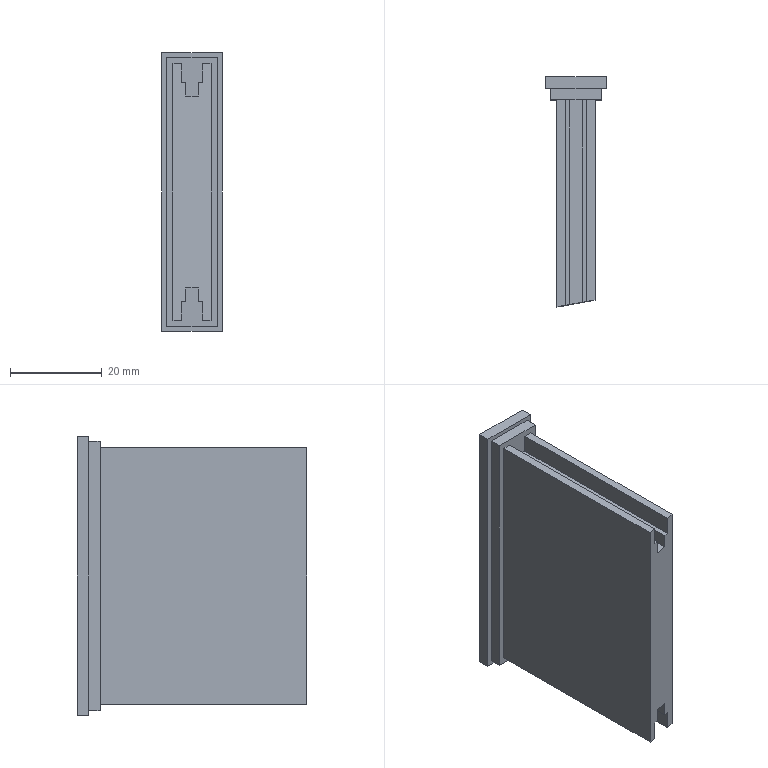Part | SolidWorks | features ICE 3, Extrusion 1 | 1 solid | 32 faces | box 13.06 x 50 x 60.56 mm | volume 21649 mm3 | plane 32
STEP:
#1=CARTESIAN_POINT('',(-2.36,45.,-27.89));
#2=VERTEX_POINT('',#1);
#3=CARTESIAN_POINT('',(-2.36,0.3139,-27.89));
#4=VERTEX_POINT('',#3);
#5=CARTESIAN_POINT('',(-2.36,45.,-27.89));
#6=DIRECTION('',(0.,-1.,0.));
#7=VECTOR('',#6,1000.);
#8=LINE('',#5,#7);
#9=EDGE_CURVE('',#2,#4,#8,.T.);
#10=ORIENTED_EDGE('',*,*,#9,.T.);
#11=CARTESIAN_POINT('',(-4.14,0.,-27.89));
#12=VERTEX_POINT('',#11);
#13=CARTESIAN_POINT('',(4.14,1.46,-27.89));
#14=DIRECTION('',(-0.9848,-0.1736,0.));
#15=VECTOR('',#14,1000.);
#16=LINE('',#13,#15);
#17=EDGE_CURVE('',#4,#12,#16,.T.);
#18=ORIENTED_EDGE('',*,*,#17,.T.);
#19=CARTESIAN_POINT('',(-4.14,45.,-27.89));
#20=VERTEX_POINT('',#19);
#21=CARTESIAN_POINT('',(-4.14,45.,-27.89));
#22=DIRECTION('',(0.,-1.,0.));
#23=VECTOR('',#22,1000.);
#24=LINE('',#21,#23);
#25=EDGE_CURVE('',#20,#12,#24,.T.);
#26=ORIENTED_EDGE('',*,*,#25,.F.);
#27=CARTESIAN_POINT('',(-2.36,45.,-27.89));
#28=DIRECTION('',(-1.,0.,0.));
#29=VECTOR('',#28,1000.);
#30=LINE('',#27,#29);
#31=EDGE_CURVE('',#2,#20,#30,.T.);
#32=ORIENTED_EDGE('',*,*,#31,.F.);
#33=EDGE_LOOP('',(#10,#18,#26,#32));
#34=FACE_OUTER_BOUND('',#33,.T.);
#35=CARTESIAN_POINT('',(-2.36,45.,-27.89));
#36=DIRECTION('',(0.,0.,1.));
#37=DIRECTION('',(1.,0.,0.));
#38=AXIS2_PLACEMENT_3D('',#35,#36,#37);
#39=PLANE('',#38);
#40=ADVANCED_FACE('',(#34),#39,.F.);
#41=CARTESIAN_POINT('',(-4.14,0.,27.89));
#42=VERTEX_POINT('',#41);
#43=CARTESIAN_POINT('',(-4.14,0.,-27.89));
#44=DIRECTION('',(0.,0.,1.));
#45=VECTOR('',#44,1000.);
#46=LINE('',#43,#45);
#47=EDGE_CURVE('',#12,#42,#46,.T.);
#48=ORIENTED_EDGE('',*,*,#47,.T.);
#49=CARTESIAN_POINT('',(-4.14,45.,27.89));
#50=VERTEX_POINT('',#49);
#51=CARTESIAN_POINT('',(-4.14,45.,27.89));
#52=DIRECTION('',(0.,-1.,0.));
#53=VECTOR('',#52,1000.);
#54=LINE('',#51,#53);
#55=EDGE_CURVE('',#50,#42,#54,.T.);
#56=ORIENTED_EDGE('',*,*,#55,.F.);
#57=CARTESIAN_POINT('',(-4.14,45.,-27.89));
#58=DIRECTION('',(0.,0.,1.));
#59=VECTOR('',#58,1000.);
#60=LINE('',#57,#59);
#61=EDGE_CURVE('',#20,#50,#60,.T.);
#62=ORIENTED_EDGE('',*,*,#61,.F.);
#63=ORIENTED_EDGE('',*,*,#25,.T.);
#64=EDGE_LOOP('',(#48,#56,#62,#63));
#65=FACE_OUTER_BOUND('',#64,.T.);
#66=CARTESIAN_POINT('',(-4.14,45.,-27.89));
#67=DIRECTION('',(1.,0.,0.));
#68=DIRECTION('',(0.,0.,-1.));
#69=AXIS2_PLACEMENT_3D('',#66,#67,#68);
#70=PLANE('',#69);
#71=ADVANCED_FACE('',(#65),#70,.F.);
#72=ORIENTED_EDGE('',*,*,#55,.T.);
#73=CARTESIAN_POINT('',(-2.36,0.3139,27.89));
#74=VERTEX_POINT('',#73);
#75=CARTESIAN_POINT('',(4.14,1.46,27.89));
#76=DIRECTION('',(-0.9848,-0.1736,0.));
#77=VECTOR('',#76,1000.);
#78=LINE('',#75,#77);
#79=EDGE_CURVE('',#74,#42,#78,.T.);
#80=ORIENTED_EDGE('',*,*,#79,.F.);
#81=CARTESIAN_POINT('',(-2.36,45.,27.89));
#82=VERTEX_POINT('',#81);
#83=CARTESIAN_POINT('',(-2.36,45.,27.89));
#84=DIRECTION('',(0.,-1.,0.));
#85=VECTOR('',#84,1000.);
#86=LINE('',#83,#85);
#87=EDGE_CURVE('',#82,#74,#86,.T.);
#88=ORIENTED_EDGE('',*,*,#87,.F.);
#89=CARTESIAN_POINT('',(-4.14,45.,27.89));
#90=DIRECTION('',(1.,0.,0.));
#91=VECTOR('',#90,1000.);
#92=LINE('',#89,#91);
#93=EDGE_CURVE('',#50,#82,#92,.T.);
#94=ORIENTED_EDGE('',*,*,#93,.F.);
#95=EDGE_LOOP('',(#72,#80,#88,#94));
#96=FACE_OUTER_BOUND('',#95,.T.);
#97=CARTESIAN_POINT('',(-4.14,45.,27.89));
#98=DIRECTION('',(0.,0.,-1.));
#99=DIRECTION('',(-1.,0.,0.));
#100=AXIS2_PLACEMENT_3D('',#97,#98,#99);
#101=PLANE('',#100);
#102=ADVANCED_FACE('',(#96),#101,.F.);
#103=ORIENTED_EDGE('',*,*,#87,.T.);
#104=CARTESIAN_POINT('',(-2.36,0.3139,23.89));
#105=VERTEX_POINT('',#104);
#106=CARTESIAN_POINT('',(-2.36,0.3139,27.89));
#107=DIRECTION('',(0.,0.,-1.));
#108=VECTOR('',#107,1000.);
#109=LINE('',#106,#108);
#110=EDGE_CURVE('',#74,#105,#109,.T.);
#111=ORIENTED_EDGE('',*,*,#110,.T.);
#112=CARTESIAN_POINT('',(-2.36,45.,23.89));
#113=VERTEX_POINT('',#112);
#114=CARTESIAN_POINT('',(-2.36,45.,23.89));
#115=DIRECTION('',(0.,-1.,0.));
#116=VECTOR('',#115,1000.);
#117=LINE('',#114,#116);
#118=EDGE_CURVE('',#113,#105,#117,.T.);
#119=ORIENTED_EDGE('',*,*,#118,.F.);
#120=CARTESIAN_POINT('',(-2.36,45.,27.89));
#121=DIRECTION('',(0.,0.,-1.));
#122=VECTOR('',#121,1000.);
#123=LINE('',#120,#122);
#124=EDGE_CURVE('',#82,#113,#123,.T.);
#125=ORIENTED_EDGE('',*,*,#124,.F.);
#126=EDGE_LOOP('',(#103,#111,#119,#125));
#127=FACE_OUTER_BOUND('',#126,.T.);
#128=CARTESIAN_POINT('',(-2.36,45.,27.89));
#129=DIRECTION('',(-1.,0.,0.));
#130=DIRECTION('',(0.,0.,1.));
#131=AXIS2_PLACEMENT_3D('',#128,#129,#130);
#132=PLANE('',#131);
#133=ADVANCED_FACE('',(#127),#132,.F.);
#134=ORIENTED_EDGE('',*,*,#118,.T.);
#135=CARTESIAN_POINT('',(-1.36,0.4902,23.89));
#136=VERTEX_POINT('',#135);
#137=CARTESIAN_POINT('',(5.282,1.661,23.89));
#138=DIRECTION('',(0.9848,0.1736,0.));
#139=VECTOR('',#138,1000.);
#140=LINE('',#137,#139);
#141=EDGE_CURVE('',#105,#136,#140,.T.);
#142=ORIENTED_EDGE('',*,*,#141,.T.);
#143=CARTESIAN_POINT('',(-1.36,45.,23.89));
#144=VERTEX_POINT('',#143);
#145=CARTESIAN_POINT('',(-1.36,45.,23.89));
#146=DIRECTION('',(0.,-1.,0.));
#147=VECTOR('',#146,1000.);
#148=LINE('',#145,#147);
#149=EDGE_CURVE('',#144,#136,#148,.T.);
#150=ORIENTED_EDGE('',*,*,#149,.F.);
#151=CARTESIAN_POINT('',(-2.36,45.,23.89));
#152=DIRECTION('',(1.,0.,0.));
#153=VECTOR('',#152,1000.);
#154=LINE('',#151,#153);
#155=EDGE_CURVE('',#113,#144,#154,.T.);
#156=ORIENTED_EDGE('',*,*,#155,.F.);
#157=EDGE_LOOP('',(#134,#142,#150,#156));
#158=FACE_OUTER_BOUND('',#157,.T.);
#159=CARTESIAN_POINT('',(-2.36,45.,23.89));
#160=DIRECTION('',(0.,0.,-1.));
#161=DIRECTION('',(-1.,0.,0.));
#162=AXIS2_PLACEMENT_3D('',#159,#160,#161);
#163=PLANE('',#162);
#164=ADVANCED_FACE('',(#158),#163,.F.);
#165=ORIENTED_EDGE('',*,*,#149,.T.);
#166=CARTESIAN_POINT('',(-1.36,0.4902,20.89));
#167=VERTEX_POINT('',#166);
#168=CARTESIAN_POINT('',(-1.36,0.4902,23.89));
#169=DIRECTION('',(0.,0.,-1.));
#170=VECTOR('',#169,1000.);
#171=LINE('',#168,#170);
#172=EDGE_CURVE('',#136,#167,#171,.T.);
#173=ORIENTED_EDGE('',*,*,#172,.T.);
#174=CARTESIAN_POINT('',(-1.36,45.,20.89));
#175=VERTEX_POINT('',#174);
#176=CARTESIAN_POINT('',(-1.36,45.,20.89));
#177=DIRECTION('',(0.,-1.,0.));
#178=VECTOR('',#177,1000.);
#179=LINE('',#176,#178);
#180=EDGE_CURVE('',#175,#167,#179,.T.);
#181=ORIENTED_EDGE('',*,*,#180,.F.);
#182=CARTESIAN_POINT('',(-1.36,45.,23.89));
#183=DIRECTION('',(0.,0.,-1.));
#184=VECTOR('',#183,1000.);
#185=LINE('',#182,#184);
#186=EDGE_CURVE('',#144,#175,#185,.T.);
#187=ORIENTED_EDGE('',*,*,#186,.F.);
#188=EDGE_LOOP('',(#165,#173,#181,#187));
#189=FACE_OUTER_BOUND('',#188,.T.);
#190=CARTESIAN_POINT('',(-1.36,45.,23.89));
#191=DIRECTION('',(-1.,0.,0.));
#192=DIRECTION('',(0.,0.,1.));
#193=AXIS2_PLACEMENT_3D('',#190,#191,#192);
#194=PLANE('',#193);
#195=ADVANCED_FACE('',(#189),#194,.F.);
#196=ORIENTED_EDGE('',*,*,#180,.T.);
#197=CARTESIAN_POINT('',(1.36,0.9698,20.89));
#198=VERTEX_POINT('',#197);
#199=CARTESIAN_POINT('',(6.252,1.832,20.89));
#200=DIRECTION('',(0.9848,0.1736,0.));
#201=VECTOR('',#200,1000.);
#202=LINE('',#199,#201);
#203=EDGE_CURVE('',#167,#198,#202,.T.);
#204=ORIENTED_EDGE('',*,*,#203,.T.);
#205=CARTESIAN_POINT('',(1.36,45.,20.89));
#206=VERTEX_POINT('',#205);
#207=CARTESIAN_POINT('',(1.36,45.,20.89));
#208=DIRECTION('',(0.,-1.,0.));
#209=VECTOR('',#208,1000.);
#210=LINE('',#207,#209);
#211=EDGE_CURVE('',#206,#198,#210,.T.);
#212=ORIENTED_EDGE('',*,*,#211,.F.);
#213=CARTESIAN_POINT('',(-1.36,45.,20.89));
#214=DIRECTION('',(1.,0.,0.));
#215=VECTOR('',#214,1000.);
#216=LINE('',#213,#215);
#217=EDGE_CURVE('',#175,#206,#216,.T.);
#218=ORIENTED_EDGE('',*,*,#217,.F.);
#219=EDGE_LOOP('',(#196,#204,#212,#218));
#220=FACE_OUTER_BOUND('',#219,.T.);
#221=CARTESIAN_POINT('',(-1.36,45.,20.89));
#222=DIRECTION('',(0.,0.,-1.));
#223=DIRECTION('',(-1.,0.,0.));
#224=AXIS2_PLACEMENT_3D('',#221,#222,#223);
#225=PLANE('',#224);
#226=ADVANCED_FACE('',(#220),#225,.F.);
#227=ORIENTED_EDGE('',*,*,#211,.T.);
#228=CARTESIAN_POINT('',(1.36,0.9698,23.89));
#229=VERTEX_POINT('',#228);
#230=CARTESIAN_POINT('',(1.36,0.9698,20.89));
#231=DIRECTION('',(0.,0.,1.));
#232=VECTOR('',#231,1000.);
#233=LINE('',#230,#232);
#234=EDGE_CURVE('',#198,#229,#233,.T.);
#235=ORIENTED_EDGE('',*,*,#234,.T.);
#236=CARTESIAN_POINT('',(1.36,45.,23.89));
#237=VERTEX_POINT('',#236);
#238=CARTESIAN_POINT('',(1.36,45.,23.89));
#239=DIRECTION('',(0.,-1.,0.));
#240=VECTOR('',#239,1000.);
#241=LINE('',#238,#240);
#242=EDGE_CURVE('',#237,#229,#241,.T.);
#243=ORIENTED_EDGE('',*,*,#242,.F.);
#244=CARTESIAN_POINT('',(1.36,45.,20.89));
#245=DIRECTION('',(0.,0.,1.));
#246=VECTOR('',#245,1000.);
#247=LINE('',#244,#246);
#248=EDGE_CURVE('',#206,#237,#247,.T.);
#249=ORIENTED_EDGE('',*,*,#248,.F.);
#250=EDGE_LOOP('',(#227,#235,#243,#249));
#251=FACE_OUTER_BOUND('',#250,.T.);
#252=CARTESIAN_POINT('',(1.36,45.,20.89));
#253=DIRECTION('',(1.,0.,0.));
#254=DIRECTION('',(0.,0.,-1.));
#255=AXIS2_PLACEMENT_3D('',#252,#253,#254);
#256=PLANE('',#255);
#257=ADVANCED_FACE('',(#251),#256,.F.);
#258=ORIENTED_EDGE('',*,*,#242,.T.);
#259=CARTESIAN_POINT('',(2.36,1.146,23.89));
#260=VERTEX_POINT('',#259);
#261=CARTESIAN_POINT('',(8.89,2.297,23.89));
#262=DIRECTION('',(0.9848,0.1736,0.));
#263=VECTOR('',#262,1000.);
#264=LINE('',#261,#263);
#265=EDGE_CURVE('',#229,#260,#264,.T.);
#266=ORIENTED_EDGE('',*,*,#265,.T.);
#267=CARTESIAN_POINT('',(2.36,45.,23.89));
#268=VERTEX_POINT('',#267);
#269=CARTESIAN_POINT('',(2.36,45.,23.89));
#270=DIRECTION('',(0.,-1.,0.));
#271=VECTOR('',#270,1000.);
#272=LINE('',#269,#271);
#273=EDGE_CURVE('',#268,#260,#272,.T.);
#274=ORIENTED_EDGE('',*,*,#273,.F.);
#275=CARTESIAN_POINT('',(1.36,45.,23.89));
#276=DIRECTION('',(1.,0.,0.));
#277=VECTOR('',#276,1000.);
#278=LINE('',#275,#277);
#279=EDGE_CURVE('',#237,#268,#278,.T.);
#280=ORIENTED_EDGE('',*,*,#279,.F.);
#281=EDGE_LOOP('',(#258,#266,#274,#280));
#282=FACE_OUTER_BOUND('',#281,.T.);
#283=CARTESIAN_POINT('',(1.36,45.,23.89));
#284=DIRECTION('',(0.,0.,-1.));
#285=DIRECTION('',(-1.,0.,0.));
#286=AXIS2_PLACEMENT_3D('',#283,#284,#285);
#287=PLANE('',#286);
#288=ADVANCED_FACE('',(#282),#287,.F.);
#289=ORIENTED_EDGE('',*,*,#273,.T.);
#290=CARTESIAN_POINT('',(2.36,1.146,27.89));
#291=VERTEX_POINT('',#290);
#292=CARTESIAN_POINT('',(2.36,1.146,23.89));
#293=DIRECTION('',(0.,0.,1.));
#294=VECTOR('',#293,1000.);
#295=LINE('',#292,#294);
#296=EDGE_CURVE('',#260,#291,#295,.T.);
#297=ORIENTED_EDGE('',*,*,#296,.T.);
#298=CARTESIAN_POINT('',(2.36,45.,27.89));
#299=VERTEX_POINT('',#298);
#300=CARTESIAN_POINT('',(2.36,45.,27.89));
#301=DIRECTION('',(0.,-1.,0.));
#302=VECTOR('',#301,1000.);
#303=LINE('',#300,#302);
#304=EDGE_CURVE('',#299,#291,#303,.T.);
#305=ORIENTED_EDGE('',*,*,#304,.F.);
#306=CARTESIAN_POINT('',(2.36,45.,23.89));
#307=DIRECTION('',(0.,0.,1.));
#308=VECTOR('',#307,1000.);
#309=LINE('',#306,#308);
#310=EDGE_CURVE('',#268,#299,#309,.T.);
#311=ORIENTED_EDGE('',*,*,#310,.F.);
#312=EDGE_LOOP('',(#289,#297,#305,#311));
#313=FACE_OUTER_BOUND('',#312,.T.);
#314=CARTESIAN_POINT('',(2.36,45.,23.89));
#315=DIRECTION('',(1.,0.,0.));
#316=DIRECTION('',(0.,0.,-1.));
#317=AXIS2_PLACEMENT_3D('',#314,#315,#316);
#318=PLANE('',#317);
#319=ADVANCED_FACE('',(#313),#318,.F.);
#320=ORIENTED_EDGE('',*,*,#304,.T.);
#321=CARTESIAN_POINT('',(4.14,1.46,27.89));
#322=VERTEX_POINT('',#321);
#323=CARTESIAN_POINT('',(4.14,1.46,27.89));
#324=DIRECTION('',(-0.9848,-0.1736,0.));
#325=VECTOR('',#324,1000.);
#326=LINE('',#323,#325);
#327=EDGE_CURVE('',#322,#291,#326,.T.);
#328=ORIENTED_EDGE('',*,*,#327,.F.);
#329=CARTESIAN_POINT('',(4.14,45.,27.89));
#330=VERTEX_POINT('',#329);
#331=CARTESIAN_POINT('',(4.14,45.,27.89));
#332=DIRECTION('',(0.,-1.,0.));
#333=VECTOR('',#332,1000.);
#334=LINE('',#331,#333);
#335=EDGE_CURVE('',#330,#322,#334,.T.);
#336=ORIENTED_EDGE('',*,*,#335,.F.);
#337=CARTESIAN_POINT('',(2.36,45.,27.89));
#338=DIRECTION('',(1.,0.,0.));
#339=VECTOR('',#338,1000.);
#340=LINE('',#337,#339);
#341=EDGE_CURVE('',#299,#330,#340,.T.);
#342=ORIENTED_EDGE('',*,*,#341,.F.);
#343=EDGE_LOOP('',(#320,#328,#336,#342));
#344=FACE_OUTER_BOUND('',#343,.T.);
#345=CARTESIAN_POINT('',(2.36,45.,27.89));
#346=DIRECTION('',(0.,0.,-1.));
#347=DIRECTION('',(-1.,0.,0.));
#348=AXIS2_PLACEMENT_3D('',#345,#346,#347);
#349=PLANE('',#348);
#350=ADVANCED_FACE('',(#344),#349,.F.);
#351=ORIENTED_EDGE('',*,*,#335,.T.);
#352=CARTESIAN_POINT('',(4.14,1.46,-27.89));
#353=VERTEX_POINT('',#352);
#354=CARTESIAN_POINT('',(4.14,1.46,-27.89));
#355=DIRECTION('',(0.,0.,1.));
#356=VECTOR('',#355,1000.);
#357=LINE('',#354,#356);
#358=EDGE_CURVE('',#353,#322,#357,.T.);
#359=ORIENTED_EDGE('',*,*,#358,.F.);
#360=CARTESIAN_POINT('',(4.14,45.,-27.89));
#361=VERTEX_POINT('',#360);
#362=CARTESIAN_POINT('',(4.14,45.,-27.89));
#363=DIRECTION('',(0.,-1.,0.));
#364=VECTOR('',#363,1000.);
#365=LINE('',#362,#364);
#366=EDGE_CURVE('',#361,#353,#365,.T.);
#367=ORIENTED_EDGE('',*,*,#366,.F.);
#368=CARTESIAN_POINT('',(4.14,45.,27.89));
#369=DIRECTION('',(0.,0.,-1.));
#370=VECTOR('',#369,1000.);
#371=LINE('',#368,#370);
#372=EDGE_CURVE('',#330,#361,#371,.T.);
#373=ORIENTED_EDGE('',*,*,#372,.F.);
#374=EDGE_LOOP('',(#351,#359,#367,#373));
#375=FACE_OUTER_BOUND('',#374,.T.);
#376=CARTESIAN_POINT('',(4.14,45.,27.89));
#377=DIRECTION('',(-1.,0.,0.));
#378=DIRECTION('',(0.,0.,1.));
#379=AXIS2_PLACEMENT_3D('',#376,#377,#378);
#380=PLANE('',#379);
#381=ADVANCED_FACE('',(#375),#380,.F.);
#382=ORIENTED_EDGE('',*,*,#366,.T.);
#383=CARTESIAN_POINT('',(2.36,1.146,-27.89));
#384=VERTEX_POINT('',#383);
#385=CARTESIAN_POINT('',(4.14,1.46,-27.89));
#386=DIRECTION('',(-0.9848,-0.1736,0.));
#387=VECTOR('',#386,1000.);
#388=LINE('',#385,#387);
#389=EDGE_CURVE('',#353,#384,#388,.T.);
#390=ORIENTED_EDGE('',*,*,#389,.T.);
#391=CARTESIAN_POINT('',(2.36,45.,-27.89));
#392=VERTEX_POINT('',#391);
#393=CARTESIAN_POINT('',(2.36,45.,-27.89));
#394=DIRECTION('',(0.,-1.,0.));
#395=VECTOR('',#394,1000.);
#396=LINE('',#393,#395);
#397=EDGE_CURVE('',#392,#384,#396,.T.);
#398=ORIENTED_EDGE('',*,*,#397,.F.);
#399=CARTESIAN_POINT('',(4.14,45.,-27.89));
#400=DIRECTION('',(-1.,0.,0.));
#401=VECTOR('',#400,1000.);
#402=LINE('',#399,#401);
#403=EDGE_CURVE('',#361,#392,#402,.T.);
#404=ORIENTED_EDGE('',*,*,#403,.F.);
#405=EDGE_LOOP('',(#382,#390,#398,#404));
#406=FACE_OUTER_BOUND('',#405,.T.);
#407=CARTESIAN_POINT('',(4.14,45.,-27.89));
#408=DIRECTION('',(0.,0.,1.));
#409=DIRECTION('',(1.,0.,0.));
#410=AXIS2_PLACEMENT_3D('',#407,#408,#409);
#411=PLANE('',#410);
#412=ADVANCED_FACE('',(#406),#411,.F.);
#413=ORIENTED_EDGE('',*,*,#397,.T.);
#414=CARTESIAN_POINT('',(2.36,1.146,-23.89));
#415=VERTEX_POINT('',#414);
#416=CARTESIAN_POINT('',(2.36,1.146,-27.89));
#417=DIRECTION('',(0.,0.,1.));
#418=VECTOR('',#417,1000.);
#419=LINE('',#416,#418);
#420=EDGE_CURVE('',#384,#415,#419,.T.);
#421=ORIENTED_EDGE('',*,*,#420,.T.);
#422=CARTESIAN_POINT('',(2.36,45.,-23.89));
#423=VERTEX_POINT('',#422);
#424=CARTESIAN_POINT('',(2.36,45.,-23.89));
#425=DIRECTION('',(0.,-1.,0.));
#426=VECTOR('',#425,1000.);
#427=LINE('',#424,#426);
#428=EDGE_CURVE('',#423,#415,#427,.T.);
#429=ORIENTED_EDGE('',*,*,#428,.F.);
#430=CARTESIAN_POINT('',(2.36,45.,-27.89));
#431=DIRECTION('',(0.,0.,1.));
#432=VECTOR('',#431,1000.);
#433=LINE('',#430,#432);
#434=EDGE_CURVE('',#392,#423,#433,.T.);
#435=ORIENTED_EDGE('',*,*,#434,.F.);
#436=EDGE_LOOP('',(#413,#421,#429,#435));
#437=FACE_OUTER_BOUND('',#436,.T.);
#438=CARTESIAN_POINT('',(2.36,45.,-27.89));
#439=DIRECTION('',(1.,0.,0.));
#440=DIRECTION('',(0.,0.,-1.));
#441=AXIS2_PLACEMENT_3D('',#438,#439,#440);
#442=PLANE('',#441);
#443=ADVANCED_FACE('',(#437),#442,.F.);
#444=ORIENTED_EDGE('',*,*,#428,.T.);
#445=CARTESIAN_POINT('',(1.36,0.9698,-23.89));
#446=VERTEX_POINT('',#445);
#447=CARTESIAN_POINT('',(9.859,2.468,-23.89));
#448=DIRECTION('',(-0.9848,-0.1736,0.));
#449=VECTOR('',#448,1000.);
#450=LINE('',#447,#449);
#451=EDGE_CURVE('',#415,#446,#450,.T.);
#452=ORIENTED_EDGE('',*,*,#451,.T.);
#453=CARTESIAN_POINT('',(1.36,45.,-23.89));
#454=VERTEX_POINT('',#453);
#455=CARTESIAN_POINT('',(1.36,45.,-23.89));
#456=DIRECTION('',(0.,-1.,0.));
#457=VECTOR('',#456,1000.);
#458=LINE('',#455,#457);
#459=EDGE_CURVE('',#454,#446,#458,.T.);
#460=ORIENTED_EDGE('',*,*,#459,.F.);
#461=CARTESIAN_POINT('',(2.36,45.,-23.89));
#462=DIRECTION('',(-1.,0.,0.));
#463=VECTOR('',#462,1000.);
#464=LINE('',#461,#463);
#465=EDGE_CURVE('',#423,#454,#464,.T.);
#466=ORIENTED_EDGE('',*,*,#465,.F.);
#467=EDGE_LOOP('',(#444,#452,#460,#466));
#468=FACE_OUTER_BOUND('',#467,.T.);
#469=CARTESIAN_POINT('',(2.36,45.,-23.89));
#470=DIRECTION('',(0.,0.,1.));
#471=DIRECTION('',(1.,0.,0.));
#472=AXIS2_PLACEMENT_3D('',#469,#470,#471);
#473=PLANE('',#472);
#474=ADVANCED_FACE('',(#468),#473,.F.);
#475=ORIENTED_EDGE('',*,*,#459,.T.);
#476=CARTESIAN_POINT('',(1.36,0.9698,-20.89));
#477=VERTEX_POINT('',#476);
#478=CARTESIAN_POINT('',(1.36,0.9698,-23.89));
#479=DIRECTION('',(0.,0.,1.));
#480=VECTOR('',#479,1000.);
#481=LINE('',#478,#480);
#482=EDGE_CURVE('',#446,#477,#481,.T.);
#483=ORIENTED_EDGE('',*,*,#482,.T.);
#484=CARTESIAN_POINT('',(1.36,45.,-20.89));
#485=VERTEX_POINT('',#484);
#486=CARTESIAN_POINT('',(1.36,45.,-20.89));
#487=DIRECTION('',(0.,-1.,0.));
#488=VECTOR('',#487,1000.);
#489=LINE('',#486,#488);
#490=EDGE_CURVE('',#485,#477,#489,.T.);
#491=ORIENTED_EDGE('',*,*,#490,.F.);
#492=CARTESIAN_POINT('',(1.36,45.,-23.89));
#493=DIRECTION('',(0.,0.,1.));
#494=VECTOR('',#493,1000.);
#495=LINE('',#492,#494);
#496=EDGE_CURVE('',#454,#485,#495,.T.);
#497=ORIENTED_EDGE('',*,*,#496,.F.);
#498=EDGE_LOOP('',(#475,#483,#491,#497));
#499=FACE_OUTER_BOUND('',#498,.T.);
#500=CARTESIAN_POINT('',(1.36,45.,-23.89));
#501=DIRECTION('',(1.,0.,0.));
#502=DIRECTION('',(0.,0.,-1.));
#503=AXIS2_PLACEMENT_3D('',#500,#501,#502);
#504=PLANE('',#503);
#505=ADVANCED_FACE('',(#499),#504,.F.);
#506=ORIENTED_EDGE('',*,*,#490,.T.);
#507=CARTESIAN_POINT('',(-1.36,0.4902,-20.89));
#508=VERTEX_POINT('',#507);
#509=CARTESIAN_POINT('',(8.89,2.297,-20.89));
#510=DIRECTION('',(-0.9848,-0.1736,0.));
#511=VECTOR('',#510,1000.);
#512=LINE('',#509,#511);
#513=EDGE_CURVE('',#477,#508,#512,.T.);
#514=ORIENTED_EDGE('',*,*,#513,.T.);
#515=CARTESIAN_POINT('',(-1.36,45.,-20.89));
#516=VERTEX_POINT('',#515);
#517=CARTESIAN_POINT('',(-1.36,45.,-20.89));
#518=DIRECTION('',(0.,-1.,0.));
#519=VECTOR('',#518,1000.);
#520=LINE('',#517,#519);
#521=EDGE_CURVE('',#516,#508,#520,.T.);
#522=ORIENTED_EDGE('',*,*,#521,.F.);
#523=CARTESIAN_POINT('',(1.36,45.,-20.89));
#524=DIRECTION('',(-1.,0.,0.));
#525=VECTOR('',#524,1000.);
#526=LINE('',#523,#525);
#527=EDGE_CURVE('',#485,#516,#526,.T.);
#528=ORIENTED_EDGE('',*,*,#527,.F.);
#529=EDGE_LOOP('',(#506,#514,#522,#528));
#530=FACE_OUTER_BOUND('',#529,.T.);
#531=CARTESIAN_POINT('',(1.36,45.,-20.89));
#532=DIRECTION('',(0.,0.,1.));
#533=DIRECTION('',(1.,0.,0.));
#534=AXIS2_PLACEMENT_3D('',#531,#532,#533);
#535=PLANE('',#534);
#536=ADVANCED_FACE('',(#530),#535,.F.);
#537=ORIENTED_EDGE('',*,*,#521,.T.);
#538=CARTESIAN_POINT('',(-1.36,0.4902,-23.89));
#539=VERTEX_POINT('',#538);
#540=CARTESIAN_POINT('',(-1.36,0.4902,-20.89));
#541=DIRECTION('',(0.,0.,-1.));
#542=VECTOR('',#541,1000.);
#543=LINE('',#540,#542);
#544=EDGE_CURVE('',#508,#539,#543,.T.);
#545=ORIENTED_EDGE('',*,*,#544,.T.);
#546=CARTESIAN_POINT('',(-1.36,45.,-23.89));
#547=VERTEX_POINT('',#546);
#548=CARTESIAN_POINT('',(-1.36,45.,-23.89));
#549=DIRECTION('',(0.,-1.,0.));
#550=VECTOR('',#549,1000.);
#551=LINE('',#548,#550);
#552=EDGE_CURVE('',#547,#539,#551,.T.);
#553=ORIENTED_EDGE('',*,*,#552,.F.);
#554=CARTESIAN_POINT('',(-1.36,45.,-20.89));
#555=DIRECTION('',(0.,0.,-1.));
#556=VECTOR('',#555,1000.);
#557=LINE('',#554,#556);
#558=EDGE_CURVE('',#516,#547,#557,.T.);
#559=ORIENTED_EDGE('',*,*,#558,.F.);
#560=EDGE_LOOP('',(#537,#545,#553,#559));
#561=FACE_OUTER_BOUND('',#560,.T.);
#562=CARTESIAN_POINT('',(-1.36,45.,-20.89));
#563=DIRECTION('',(-1.,0.,0.));
#564=DIRECTION('',(0.,0.,1.));
#565=AXIS2_PLACEMENT_3D('',#562,#563,#564);
#566=PLANE('',#565);
#567=ADVANCED_FACE('',(#561),#566,.F.);
#568=ORIENTED_EDGE('',*,*,#552,.T.);
#569=CARTESIAN_POINT('',(-2.36,0.3139,-23.89));
#570=VERTEX_POINT('',#569);
#571=CARTESIAN_POINT('',(6.252,1.832,-23.89));
#572=DIRECTION('',(-0.9848,-0.1736,0.));
#573=VECTOR('',#572,1000.);
#574=LINE('',#571,#573);
#575=EDGE_CURVE('',#539,#570,#574,.T.);
#576=ORIENTED_EDGE('',*,*,#575,.T.);
#577=CARTESIAN_POINT('',(-2.36,45.,-23.89));
#578=VERTEX_POINT('',#577);
#579=CARTESIAN_POINT('',(-2.36,45.,-23.89));
#580=DIRECTION('',(0.,-1.,0.));
#581=VECTOR('',#580,1000.);
#582=LINE('',#579,#581);
#583=EDGE_CURVE('',#578,#570,#582,.T.);
#584=ORIENTED_EDGE('',*,*,#583,.F.);
#585=CARTESIAN_POINT('',(-1.36,45.,-23.89));
#586=DIRECTION('',(-1.,0.,0.));
#587=VECTOR('',#586,1000.);
#588=LINE('',#585,#587);
#589=EDGE_CURVE('',#547,#578,#588,.T.);
#590=ORIENTED_EDGE('',*,*,#589,.F.);
#591=EDGE_LOOP('',(#568,#576,#584,#590));
#592=FACE_OUTER_BOUND('',#591,.T.);
#593=CARTESIAN_POINT('',(-1.36,45.,-23.89));
#594=DIRECTION('',(0.,0.,1.));
#595=DIRECTION('',(1.,0.,0.));
#596=AXIS2_PLACEMENT_3D('',#593,#594,#595);
#597=PLANE('',#596);
#598=ADVANCED_FACE('',(#592),#597,.F.);
#599=ORIENTED_EDGE('',*,*,#583,.T.);
#600=CARTESIAN_POINT('',(-2.36,0.3139,-23.89));
#601=DIRECTION('',(0.,0.,-1.));
#602=VECTOR('',#601,1000.);
#603=LINE('',#600,#602);
#604=EDGE_CURVE('',#570,#4,#603,.T.);
#605=ORIENTED_EDGE('',*,*,#604,.T.);
#606=ORIENTED_EDGE('',*,*,#9,.F.);
#607=CARTESIAN_POINT('',(-2.36,45.,-23.89));
#608=DIRECTION('',(0.,0.,-1.));
#609=VECTOR('',#608,1000.);
#610=LINE('',#607,#609);
#611=EDGE_CURVE('',#578,#2,#610,.T.);
#612=ORIENTED_EDGE('',*,*,#611,.F.);
#613=EDGE_LOOP('',(#599,#605,#606,#612));
#614=FACE_OUTER_BOUND('',#613,.T.);
#615=CARTESIAN_POINT('',(-2.36,45.,-23.89));
#616=DIRECTION('',(-1.,0.,0.));
#617=DIRECTION('',(0.,0.,1.));
#618=AXIS2_PLACEMENT_3D('',#615,#616,#617);
#619=PLANE('',#618);
#620=ADVANCED_FACE('',(#614),#619,.F.);
#621=ORIENTED_EDGE('',*,*,#79,.T.);
#622=ORIENTED_EDGE('',*,*,#47,.F.);
#623=ORIENTED_EDGE('',*,*,#17,.F.);
#624=ORIENTED_EDGE('',*,*,#604,.F.);
#625=ORIENTED_EDGE('',*,*,#575,.F.);
#626=ORIENTED_EDGE('',*,*,#544,.F.);
#627=ORIENTED_EDGE('',*,*,#513,.F.);
#628=ORIENTED_EDGE('',*,*,#482,.F.);
#629=ORIENTED_EDGE('',*,*,#451,.F.);
#630=ORIENTED_EDGE('',*,*,#420,.F.);
#631=ORIENTED_EDGE('',*,*,#389,.F.);
#632=ORIENTED_EDGE('',*,*,#358,.T.);
#633=ORIENTED_EDGE('',*,*,#327,.T.);
#634=ORIENTED_EDGE('',*,*,#296,.F.);
#635=ORIENTED_EDGE('',*,*,#265,.F.);
#636=ORIENTED_EDGE('',*,*,#234,.F.);
#637=ORIENTED_EDGE('',*,*,#203,.F.);
#638=ORIENTED_EDGE('',*,*,#172,.F.);
#639=ORIENTED_EDGE('',*,*,#141,.F.);
#640=ORIENTED_EDGE('',*,*,#110,.F.);
#641=EDGE_LOOP('',(#621,#622,#623,#624,#625,#626,#627,#628,#629,#630,#631,#632,#633,#634,#635,#636,#637,#638,#639,#640));
#642=FACE_OUTER_BOUND('',#641,.T.);
#643=CARTESIAN_POINT('',(4.14,1.46,-27.89));
#644=DIRECTION('',(-0.1736,0.9848,0.));
#645=DIRECTION('',(-0.9848,-0.1736,0.));
#646=AXIS2_PLACEMENT_3D('',#643,#644,#645);
#647=PLANE('',#646);
#648=ADVANCED_FACE('',(#642),#647,.F.);
#649=CARTESIAN_POINT('',(-5.53,45.,-29.28));
#650=VERTEX_POINT('',#649);
#651=CARTESIAN_POINT('',(-5.53,45.,29.28));
#652=VERTEX_POINT('',#651);
#653=CARTESIAN_POINT('',(-5.53,45.,-29.28));
#654=DIRECTION('',(0.,0.,1.));
#655=VECTOR('',#654,1000.);
#656=LINE('',#653,#655);
#657=EDGE_CURVE('',#650,#652,#656,.T.);
#658=ORIENTED_EDGE('',*,*,#657,.F.);
#659=CARTESIAN_POINT('',(5.53,45.,-29.28));
#660=VERTEX_POINT('',#659);
#661=CARTESIAN_POINT('',(-5.53,45.,-29.28));
#662=DIRECTION('',(-1.,0.,0.));
#663=VECTOR('',#662,1000.);
#664=LINE('',#661,#663);
#665=EDGE_CURVE('',#660,#650,#664,.T.);
#666=ORIENTED_EDGE('',*,*,#665,.F.);
#667=CARTESIAN_POINT('',(5.53,45.,29.28));
#668=VERTEX_POINT('',#667);
#669=CARTESIAN_POINT('',(5.53,45.,-29.28));
#670=DIRECTION('',(0.,0.,-1.));
#671=VECTOR('',#670,1000.);
#672=LINE('',#669,#671);
#673=EDGE_CURVE('',#668,#660,#672,.T.);
#674=ORIENTED_EDGE('',*,*,#673,.F.);
#675=CARTESIAN_POINT('',(-5.53,45.,29.28));
#676=DIRECTION('',(1.,0.,0.));
#677=VECTOR('',#676,1000.);
#678=LINE('',#675,#677);
#679=EDGE_CURVE('',#652,#668,#678,.T.);
#680=ORIENTED_EDGE('',*,*,#679,.F.);
#681=EDGE_LOOP('',(#658,#666,#674,#680));
#682=FACE_OUTER_BOUND('',#681,.T.);
#683=ORIENTED_EDGE('',*,*,#611,.T.);
#684=ORIENTED_EDGE('',*,*,#31,.T.);
#685=ORIENTED_EDGE('',*,*,#61,.T.);
#686=ORIENTED_EDGE('',*,*,#93,.T.);
#687=ORIENTED_EDGE('',*,*,#124,.T.);
#688=ORIENTED_EDGE('',*,*,#155,.T.);
#689=ORIENTED_EDGE('',*,*,#186,.T.);
#690=ORIENTED_EDGE('',*,*,#217,.T.);
#691=ORIENTED_EDGE('',*,*,#248,.T.);
#692=ORIENTED_EDGE('',*,*,#279,.T.);
#693=ORIENTED_EDGE('',*,*,#310,.T.);
#694=ORIENTED_EDGE('',*,*,#341,.T.);
#695=ORIENTED_EDGE('',*,*,#372,.T.);
#696=ORIENTED_EDGE('',*,*,#403,.T.);
#697=ORIENTED_EDGE('',*,*,#434,.T.);
#698=ORIENTED_EDGE('',*,*,#465,.T.);
#699=ORIENTED_EDGE('',*,*,#496,.T.);
#700=ORIENTED_EDGE('',*,*,#527,.T.);
#701=ORIENTED_EDGE('',*,*,#558,.T.);
#702=ORIENTED_EDGE('',*,*,#589,.T.);
#703=EDGE_LOOP('',(#683,#684,#685,#686,#687,#688,#689,#690,#691,#692,#693,#694,#695,#696,#697,#698,#699,#700,#701,#702));
#704=FACE_BOUND('',#703,.T.);
#705=CARTESIAN_POINT('',(0.,45.,0.));
#706=DIRECTION('',(0.,1.,0.));
#707=DIRECTION('',(0.,0.,1.));
#708=AXIS2_PLACEMENT_3D('',#705,#706,#707);
#709=PLANE('',#708);
#710=ADVANCED_FACE('',(#682,#704),#709,.F.);
#711=ORIENTED_EDGE('',*,*,#657,.T.);
#712=CARTESIAN_POINT('',(-5.53,47.5,29.28));
#713=VERTEX_POINT('',#712);
#714=CARTESIAN_POINT('',(-5.53,47.5,29.28));
#715=DIRECTION('',(0.,-1.,0.));
#716=VECTOR('',#715,1000.);
#717=LINE('',#714,#716);
#718=EDGE_CURVE('',#713,#652,#717,.T.);
#719=ORIENTED_EDGE('',*,*,#718,.F.);
#720=CARTESIAN_POINT('',(-5.53,47.5,-29.28));
#721=VERTEX_POINT('',#720);
#722=CARTESIAN_POINT('',(-5.53,47.5,-29.28));
#723=DIRECTION('',(0.,0.,1.));
#724=VECTOR('',#723,1000.);
#725=LINE('',#722,#724);
#726=EDGE_CURVE('',#721,#713,#725,.T.);
#727=ORIENTED_EDGE('',*,*,#726,.F.);
#728=CARTESIAN_POINT('',(-5.53,47.5,-29.28));
#729=DIRECTION('',(0.,-1.,0.));
#730=VECTOR('',#729,1000.);
#731=LINE('',#728,#730);
#732=EDGE_CURVE('',#721,#650,#731,.T.);
#733=ORIENTED_EDGE('',*,*,#732,.T.);
#734=EDGE_LOOP('',(#711,#719,#727,#733));
#735=FACE_OUTER_BOUND('',#734,.T.);
#736=CARTESIAN_POINT('',(-5.53,47.5,-29.28));
#737=DIRECTION('',(1.,0.,0.));
#738=DIRECTION('',(0.,0.,-1.));
#739=AXIS2_PLACEMENT_3D('',#736,#737,#738);
#740=PLANE('',#739);
#741=ADVANCED_FACE('',(#735),#740,.F.);
#742=ORIENTED_EDGE('',*,*,#679,.T.);
#743=CARTESIAN_POINT('',(5.53,47.5,29.28));
#744=VERTEX_POINT('',#743);
#745=CARTESIAN_POINT('',(5.53,47.5,29.28));
#746=DIRECTION('',(0.,-1.,0.));
#747=VECTOR('',#746,1000.);
#748=LINE('',#745,#747);
#749=EDGE_CURVE('',#744,#668,#748,.T.);
#750=ORIENTED_EDGE('',*,*,#749,.F.);
#751=CARTESIAN_POINT('',(-5.53,47.5,29.28));
#752=DIRECTION('',(1.,0.,0.));
#753=VECTOR('',#752,1000.);
#754=LINE('',#751,#753);
#755=EDGE_CURVE('',#713,#744,#754,.T.);
#756=ORIENTED_EDGE('',*,*,#755,.F.);
#757=ORIENTED_EDGE('',*,*,#718,.T.);
#758=EDGE_LOOP('',(#742,#750,#756,#757));
#759=FACE_OUTER_BOUND('',#758,.T.);
#760=CARTESIAN_POINT('',(-5.53,47.5,29.28));
#761=DIRECTION('',(0.,0.,-1.));
#762=DIRECTION('',(-1.,0.,0.));
#763=AXIS2_PLACEMENT_3D('',#760,#761,#762);
#764=PLANE('',#763);
#765=ADVANCED_FACE('',(#759),#764,.F.);
#766=ORIENTED_EDGE('',*,*,#673,.T.);
#767=CARTESIAN_POINT('',(5.53,47.5,-29.28));
#768=VERTEX_POINT('',#767);
#769=CARTESIAN_POINT('',(5.53,47.5,-29.28));
#770=DIRECTION('',(0.,-1.,0.));
#771=VECTOR('',#770,1000.);
#772=LINE('',#769,#771);
#773=EDGE_CURVE('',#768,#660,#772,.T.);
#774=ORIENTED_EDGE('',*,*,#773,.F.);
#775=CARTESIAN_POINT('',(5.53,47.5,-29.28));
#776=DIRECTION('',(0.,0.,-1.));
#777=VECTOR('',#776,1000.);
#778=LINE('',#775,#777);
#779=EDGE_CURVE('',#744,#768,#778,.T.);
#780=ORIENTED_EDGE('',*,*,#779,.F.);
#781=ORIENTED_EDGE('',*,*,#749,.T.);
#782=EDGE_LOOP('',(#766,#774,#780,#781));
#783=FACE_OUTER_BOUND('',#782,.T.);
#784=CARTESIAN_POINT('',(5.53,47.5,-29.28));
#785=DIRECTION('',(-1.,0.,0.));
#786=DIRECTION('',(0.,0.,1.));
#787=AXIS2_PLACEMENT_3D('',#784,#785,#786);
#788=PLANE('',#787);
#789=ADVANCED_FACE('',(#783),#788,.F.);
#790=ORIENTED_EDGE('',*,*,#665,.T.);
#791=ORIENTED_EDGE('',*,*,#732,.F.);
#792=CARTESIAN_POINT('',(-5.53,47.5,-29.28));
#793=DIRECTION('',(-1.,0.,0.));
#794=VECTOR('',#793,1000.);
#795=LINE('',#792,#794);
#796=EDGE_CURVE('',#768,#721,#795,.T.);
#797=ORIENTED_EDGE('',*,*,#796,.F.);
#798=ORIENTED_EDGE('',*,*,#773,.T.);
#799=EDGE_LOOP('',(#790,#791,#797,#798));
#800=FACE_OUTER_BOUND('',#799,.T.);
#801=CARTESIAN_POINT('',(-5.53,47.5,-29.28));
#802=DIRECTION('',(0.,0.,1.));
#803=DIRECTION('',(1.,0.,0.));
#804=AXIS2_PLACEMENT_3D('',#801,#802,#803);
#805=PLANE('',#804);
#806=ADVANCED_FACE('',(#800),#805,.F.);
#807=CARTESIAN_POINT('',(-6.53,47.5,-30.28));
#808=VERTEX_POINT('',#807);
#809=CARTESIAN_POINT('',(-6.53,47.5,30.28));
#810=VERTEX_POINT('',#809);
#811=CARTESIAN_POINT('',(-6.53,47.5,30.28));
#812=DIRECTION('',(0.,0.,1.));
#813=VECTOR('',#812,1000.);
#814=LINE('',#811,#813);
#815=EDGE_CURVE('',#808,#810,#814,.T.);
#816=ORIENTED_EDGE('',*,*,#815,.F.);
#817=CARTESIAN_POINT('',(6.53,47.5,-30.28));
#818=VERTEX_POINT('',#817);
#819=CARTESIAN_POINT('',(-6.53,47.5,-30.28));
#820=DIRECTION('',(-1.,0.,0.));
#821=VECTOR('',#820,1000.);
#822=LINE('',#819,#821);
#823=EDGE_CURVE('',#818,#808,#822,.T.);
#824=ORIENTED_EDGE('',*,*,#823,.F.);
#825=CARTESIAN_POINT('',(6.53,47.5,30.28));
#826=VERTEX_POINT('',#825);
#827=CARTESIAN_POINT('',(6.53,47.5,-30.28));
#828=DIRECTION('',(0.,0.,-1.));
#829=VECTOR('',#828,1000.);
#830=LINE('',#827,#829);
#831=EDGE_CURVE('',#826,#818,#830,.T.);
#832=ORIENTED_EDGE('',*,*,#831,.F.);
#833=CARTESIAN_POINT('',(6.53,47.5,30.28));
#834=DIRECTION('',(1.,0.,0.));
#835=VECTOR('',#834,1000.);
#836=LINE('',#833,#835);
#837=EDGE_CURVE('',#810,#826,#836,.T.);
#838=ORIENTED_EDGE('',*,*,#837,.F.);
#839=EDGE_LOOP('',(#816,#824,#832,#838));
#840=FACE_OUTER_BOUND('',#839,.T.);
#841=ORIENTED_EDGE('',*,*,#726,.T.);
#842=ORIENTED_EDGE('',*,*,#755,.T.);
#843=ORIENTED_EDGE('',*,*,#779,.T.);
#844=ORIENTED_EDGE('',*,*,#796,.T.);
#845=EDGE_LOOP('',(#841,#842,#843,#844));
#846=FACE_BOUND('',#845,.T.);
#847=CARTESIAN_POINT('',(0.,47.5,0.));
#848=DIRECTION('',(0.,-1.,0.));
#849=DIRECTION('',(0.,0.,-1.));
#850=AXIS2_PLACEMENT_3D('',#847,#848,#849);
#851=PLANE('',#850);
#852=ADVANCED_FACE('',(#840,#846),#851,.T.);
#853=ORIENTED_EDGE('',*,*,#815,.T.);
#854=CARTESIAN_POINT('',(-6.53,50.,30.28));
#855=VERTEX_POINT('',#854);
#856=CARTESIAN_POINT('',(-6.53,50.,30.28));
#857=DIRECTION('',(0.,-1.,0.));
#858=VECTOR('',#857,1000.);
#859=LINE('',#856,#858);
#860=EDGE_CURVE('',#855,#810,#859,.T.);
#861=ORIENTED_EDGE('',*,*,#860,.F.);
#862=CARTESIAN_POINT('',(-6.53,50.,-30.28));
#863=VERTEX_POINT('',#862);
#864=CARTESIAN_POINT('',(-6.53,50.,30.28));
#865=DIRECTION('',(0.,0.,1.));
#866=VECTOR('',#865,1000.);
#867=LINE('',#864,#866);
#868=EDGE_CURVE('',#863,#855,#867,.T.);
#869=ORIENTED_EDGE('',*,*,#868,.F.);
#870=CARTESIAN_POINT('',(-6.53,50.,-30.28));
#871=DIRECTION('',(0.,-1.,0.));
#872=VECTOR('',#871,1000.);
#873=LINE('',#870,#872);
#874=EDGE_CURVE('',#863,#808,#873,.T.);
#875=ORIENTED_EDGE('',*,*,#874,.T.);
#876=EDGE_LOOP('',(#853,#861,#869,#875));
#877=FACE_OUTER_BOUND('',#876,.T.);
#878=CARTESIAN_POINT('',(-6.53,50.,30.28));
#879=DIRECTION('',(1.,0.,0.));
#880=DIRECTION('',(0.,0.,-1.));
#881=AXIS2_PLACEMENT_3D('',#878,#879,#880);
#882=PLANE('',#881);
#883=ADVANCED_FACE('',(#877),#882,.F.);
#884=ORIENTED_EDGE('',*,*,#837,.T.);
#885=CARTESIAN_POINT('',(6.53,50.,30.28));
#886=VERTEX_POINT('',#885);
#887=CARTESIAN_POINT('',(6.53,50.,30.28));
#888=DIRECTION('',(0.,-1.,0.));
#889=VECTOR('',#888,1000.);
#890=LINE('',#887,#889);
#891=EDGE_CURVE('',#886,#826,#890,.T.);
#892=ORIENTED_EDGE('',*,*,#891,.F.);
#893=CARTESIAN_POINT('',(6.53,50.,30.28));
#894=DIRECTION('',(1.,0.,0.));
#895=VECTOR('',#894,1000.);
#896=LINE('',#893,#895);
#897=EDGE_CURVE('',#855,#886,#896,.T.);
#898=ORIENTED_EDGE('',*,*,#897,.F.);
#899=ORIENTED_EDGE('',*,*,#860,.T.);
#900=EDGE_LOOP('',(#884,#892,#898,#899));
#901=FACE_OUTER_BOUND('',#900,.T.);
#902=CARTESIAN_POINT('',(6.53,50.,30.28));
#903=DIRECTION('',(0.,0.,-1.));
#904=DIRECTION('',(-1.,0.,0.));
#905=AXIS2_PLACEMENT_3D('',#902,#903,#904);
#906=PLANE('',#905);
#907=ADVANCED_FACE('',(#901),#906,.F.);
#908=ORIENTED_EDGE('',*,*,#831,.T.);
#909=CARTESIAN_POINT('',(6.53,50.,-30.28));
#910=VERTEX_POINT('',#909);
#911=CARTESIAN_POINT('',(6.53,50.,-30.28));
#912=DIRECTION('',(0.,-1.,0.));
#913=VECTOR('',#912,1000.);
#914=LINE('',#911,#913);
#915=EDGE_CURVE('',#910,#818,#914,.T.);
#916=ORIENTED_EDGE('',*,*,#915,.F.);
#917=CARTESIAN_POINT('',(6.53,50.,-30.28));
#918=DIRECTION('',(0.,0.,-1.));
#919=VECTOR('',#918,1000.);
#920=LINE('',#917,#919);
#921=EDGE_CURVE('',#886,#910,#920,.T.);
#922=ORIENTED_EDGE('',*,*,#921,.F.);
#923=ORIENTED_EDGE('',*,*,#891,.T.);
#924=EDGE_LOOP('',(#908,#916,#922,#923));
#925=FACE_OUTER_BOUND('',#924,.T.);
#926=CARTESIAN_POINT('',(6.53,50.,-30.28));
#927=DIRECTION('',(-1.,0.,0.));
#928=DIRECTION('',(0.,0.,1.));
#929=AXIS2_PLACEMENT_3D('',#926,#927,#928);
#930=PLANE('',#929);
#931=ADVANCED_FACE('',(#925),#930,.F.);
#932=ORIENTED_EDGE('',*,*,#823,.T.);
#933=ORIENTED_EDGE('',*,*,#874,.F.);
#934=CARTESIAN_POINT('',(-6.53,50.,-30.28));
#935=DIRECTION('',(-1.,0.,0.));
#936=VECTOR('',#935,1000.);
#937=LINE('',#934,#936);
#938=EDGE_CURVE('',#910,#863,#937,.T.);
#939=ORIENTED_EDGE('',*,*,#938,.F.);
#940=ORIENTED_EDGE('',*,*,#915,.T.);
#941=EDGE_LOOP('',(#932,#933,#939,#940));
#942=FACE_OUTER_BOUND('',#941,.T.);
#943=CARTESIAN_POINT('',(-6.53,50.,-30.28));
#944=DIRECTION('',(0.,0.,1.));
#945=DIRECTION('',(1.,0.,0.));
#946=AXIS2_PLACEMENT_3D('',#943,#944,#945);
#947=PLANE('',#946);
#948=ADVANCED_FACE('',(#942),#947,.F.);
#949=ORIENTED_EDGE('',*,*,#868,.T.);
#950=ORIENTED_EDGE('',*,*,#897,.T.);
#951=ORIENTED_EDGE('',*,*,#921,.T.);
#952=ORIENTED_EDGE('',*,*,#938,.T.);
#953=EDGE_LOOP('',(#949,#950,#951,#952));
#954=FACE_OUTER_BOUND('',#953,.T.);
#955=CARTESIAN_POINT('',(0.,50.,0.));
#956=DIRECTION('',(0.,-1.,0.));
#957=DIRECTION('',(0.,0.,-1.));
#958=AXIS2_PLACEMENT_3D('',#955,#956,#957);
#959=PLANE('',#958);
#960=ADVANCED_FACE('',(#954),#959,.F.);
#961=CLOSED_SHELL('',(#40,#71,#102,#133,#164,#195,#226,#257,#288,#319,#350,#381,#412,#443,#474,#505,#536,#567,#598,#620,#648,#710,#741,#765,#789,#806,#852,#883,#907,#931,#948,#960));
#962=MANIFOLD_SOLID_BREP('',#961);
#963=CARTESIAN_POINT('',(0.,0.,0.));
#964=DIRECTION('',(0.,0.,1.));
#965=DIRECTION('',(1.,0.,0.));
#966=AXIS2_PLACEMENT_3D('',#963,#964,#965);
#967=(LENGTH_UNIT()NAMED_UNIT(*)SI_UNIT(.MILLI.,.METRE.));
#968=UNCERTAINTY_MEASURE_WITH_UNIT(LENGTH_MEASURE(0.00001),#967,'','');
#969=(NAMED_UNIT(*)PLANE_ANGLE_UNIT()SI_UNIT($,.RADIAN.));
#970=(NAMED_UNIT(*)SI_UNIT($,.STERADIAN.)SOLID_ANGLE_UNIT());
#971=(GEOMETRIC_REPRESENTATION_CONTEXT(3)GLOBAL_UNCERTAINTY_ASSIGNED_CONTEXT((#968))GLOBAL_UNIT_ASSIGNED_CONTEXT((#967,#969,#970))REPRESENTATION_CONTEXT('',''));
#972=ADVANCED_BREP_SHAPE_REPRESENTATION('',(#962,#966),#971);